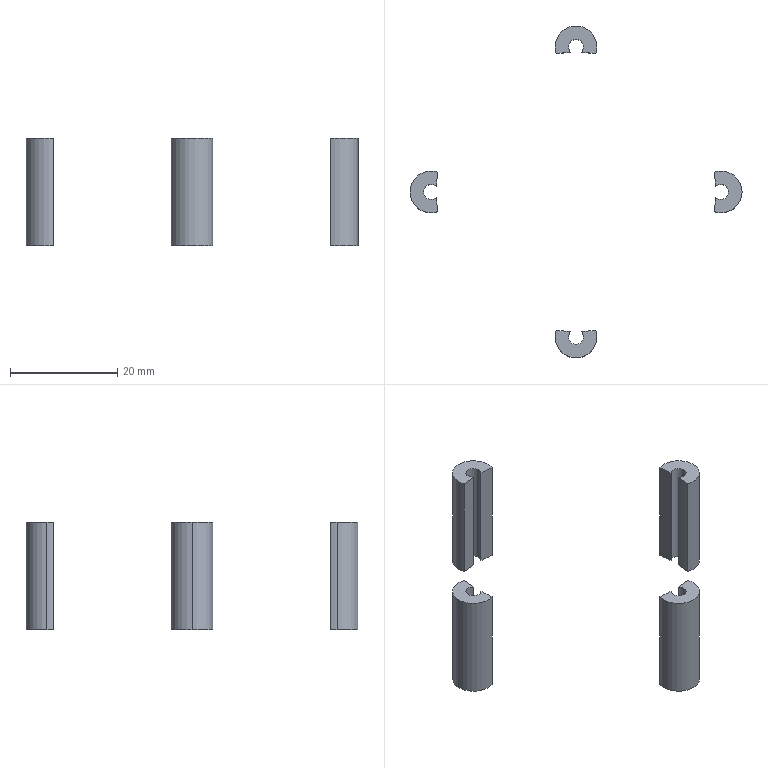Part | SolidWorks | features BaseBody 4 | 4 solids | 34 faces | box 61.8 x 61.8 x 20 mm | volume 2131 mm3 | cylinder 26 | plane 8 | commonest cylinder face diameters 2.8 x9 7.8 x9 52 x8
STEP:
#1=CARTESIAN_POINT('',(3.69,-25.737,11.));
#2=VERTEX_POINT('',#1);
#3=CARTESIAN_POINT('',(3.9,-27.,11.));
#4=VERTEX_POINT('',#3);
#5=CARTESIAN_POINT('',(0.,-27.,11.));
#6=DIRECTION('',(0.,0.,-1.));
#7=DIRECTION('',(-1.,0.,0.));
#8=AXIS2_PLACEMENT_3D('',#5,#6,#7);
#9=CIRCLE('',#8,3.9);
#10=EDGE_CURVE('',#2,#4,#9,.T.);
#11=ORIENTED_EDGE('',*,*,#10,.T.);
#12=CARTESIAN_POINT('',(3.9,-27.,-9.));
#13=VERTEX_POINT('',#12);
#14=CARTESIAN_POINT('',(3.9,-27.,-9.));
#15=DIRECTION('',(0.,0.,-1.));
#16=VECTOR('',#15,1000.);
#17=LINE('',#14,#16);
#18=EDGE_CURVE('',#4,#13,#17,.T.);
#19=ORIENTED_EDGE('',*,*,#18,.T.);
#20=CARTESIAN_POINT('',(3.69,-25.737,-9.));
#21=VERTEX_POINT('',#20);
#22=CARTESIAN_POINT('',(0.,-27.,-9.));
#23=DIRECTION('',(0.,0.,1.));
#24=DIRECTION('',(-1.,0.,0.));
#25=AXIS2_PLACEMENT_3D('',#22,#23,#24);
#26=CIRCLE('',#25,3.9);
#27=EDGE_CURVE('',#13,#21,#26,.T.);
#28=ORIENTED_EDGE('',*,*,#27,.T.);
#29=CARTESIAN_POINT('',(3.69,-25.737,-9.));
#30=DIRECTION('',(0.,0.,1.));
#31=VECTOR('',#30,1000.);
#32=LINE('',#29,#31);
#33=EDGE_CURVE('',#21,#2,#32,.T.);
#34=ORIENTED_EDGE('',*,*,#33,.T.);
#35=EDGE_LOOP('',(#11,#19,#28,#34));
#36=FACE_OUTER_BOUND('',#35,.T.);
#37=CARTESIAN_POINT('',(0.,-27.,-9.));
#38=DIRECTION('',(0.,0.,-1.));
#39=DIRECTION('',(-1.,0.,0.));
#40=AXIS2_PLACEMENT_3D('',#37,#38,#39);
#41=CYLINDRICAL_SURFACE('',#40,3.9);
#42=ADVANCED_FACE('',(#36),#41,.T.);
#43=ORIENTED_EDGE('',*,*,#18,.F.);
#44=CARTESIAN_POINT('',(-3.9,-27.,11.));
#45=VERTEX_POINT('',#44);
#46=CARTESIAN_POINT('',(0.,-27.,11.));
#47=DIRECTION('',(0.,0.,-1.));
#48=DIRECTION('',(-1.,0.,0.));
#49=AXIS2_PLACEMENT_3D('',#46,#47,#48);
#50=CIRCLE('',#49,3.9);
#51=EDGE_CURVE('',#4,#45,#50,.T.);
#52=ORIENTED_EDGE('',*,*,#51,.T.);
#53=CARTESIAN_POINT('',(-3.9,-27.,-9.));
#54=VERTEX_POINT('',#53);
#55=CARTESIAN_POINT('',(-3.9,-27.,-9.));
#56=DIRECTION('',(0.,0.,-1.));
#57=VECTOR('',#56,1000.);
#58=LINE('',#55,#57);
#59=EDGE_CURVE('',#45,#54,#58,.T.);
#60=ORIENTED_EDGE('',*,*,#59,.T.);
#61=CARTESIAN_POINT('',(0.,-27.,-9.));
#62=DIRECTION('',(0.,0.,1.));
#63=DIRECTION('',(-1.,0.,0.));
#64=AXIS2_PLACEMENT_3D('',#61,#62,#63);
#65=CIRCLE('',#64,3.9);
#66=EDGE_CURVE('',#54,#13,#65,.T.);
#67=ORIENTED_EDGE('',*,*,#66,.T.);
#68=EDGE_LOOP('',(#43,#52,#60,#67));
#69=FACE_OUTER_BOUND('',#68,.T.);
#70=CARTESIAN_POINT('',(0.,-27.,-9.));
#71=DIRECTION('',(0.,0.,-1.));
#72=DIRECTION('',(-1.,0.,0.));
#73=AXIS2_PLACEMENT_3D('',#70,#71,#72);
#74=CYLINDRICAL_SURFACE('',#73,3.9);
#75=ADVANCED_FACE('',(#69),#74,.T.);
#76=CARTESIAN_POINT('',(1.4,-27.,11.));
#77=VERTEX_POINT('',#76);
#78=CARTESIAN_POINT('',(-1.4,-27.,11.));
#79=VERTEX_POINT('',#78);
#80=CARTESIAN_POINT('',(0.,-27.,11.));
#81=DIRECTION('',(0.,0.,-1.));
#82=DIRECTION('',(-1.,0.,0.));
#83=AXIS2_PLACEMENT_3D('',#80,#81,#82);
#84=CIRCLE('',#83,1.4);
#85=EDGE_CURVE('',#77,#79,#84,.T.);
#86=ORIENTED_EDGE('',*,*,#85,.F.);
#87=CARTESIAN_POINT('',(1.4,-27.,-9.));
#88=VERTEX_POINT('',#87);
#89=CARTESIAN_POINT('',(1.4,-27.,-9.));
#90=DIRECTION('',(0.,0.,-1.));
#91=VECTOR('',#90,1000.);
#92=LINE('',#89,#91);
#93=EDGE_CURVE('',#77,#88,#92,.T.);
#94=ORIENTED_EDGE('',*,*,#93,.T.);
#95=CARTESIAN_POINT('',(-1.4,-27.,-9.));
#96=VERTEX_POINT('',#95);
#97=CARTESIAN_POINT('',(0.,-27.,-9.));
#98=DIRECTION('',(0.,0.,-1.));
#99=DIRECTION('',(-1.,0.,0.));
#100=AXIS2_PLACEMENT_3D('',#97,#98,#99);
#101=CIRCLE('',#100,1.4);
#102=EDGE_CURVE('',#88,#96,#101,.T.);
#103=ORIENTED_EDGE('',*,*,#102,.T.);
#104=CARTESIAN_POINT('',(-1.4,-27.,-9.));
#105=DIRECTION('',(0.,0.,-1.));
#106=VECTOR('',#105,1000.);
#107=LINE('',#104,#106);
#108=EDGE_CURVE('',#79,#96,#107,.T.);
#109=ORIENTED_EDGE('',*,*,#108,.F.);
#110=EDGE_LOOP('',(#86,#94,#103,#109));
#111=FACE_OUTER_BOUND('',#110,.T.);
#112=CARTESIAN_POINT('',(0.,-27.,-9.));
#113=DIRECTION('',(0.,0.,-1.));
#114=DIRECTION('',(-1.,0.,0.));
#115=AXIS2_PLACEMENT_3D('',#112,#113,#114);
#116=CYLINDRICAL_SURFACE('',#115,1.4);
#117=ADVANCED_FACE('',(#111),#116,.F.);
#118=CARTESIAN_POINT('',(-0.9613,-25.982,11.));
#119=VERTEX_POINT('',#118);
#120=CARTESIAN_POINT('',(0.,-27.,11.));
#121=DIRECTION('',(0.,0.,-1.));
#122=DIRECTION('',(-1.,0.,0.));
#123=AXIS2_PLACEMENT_3D('',#120,#121,#122);
#124=CIRCLE('',#123,1.4);
#125=EDGE_CURVE('',#79,#119,#124,.T.);
#126=ORIENTED_EDGE('',*,*,#125,.F.);
#127=ORIENTED_EDGE('',*,*,#108,.T.);
#128=CARTESIAN_POINT('',(-0.9613,-25.982,-9.));
#129=VERTEX_POINT('',#128);
#130=CARTESIAN_POINT('',(0.,-27.,-9.));
#131=DIRECTION('',(0.,0.,-1.));
#132=DIRECTION('',(-1.,0.,0.));
#133=AXIS2_PLACEMENT_3D('',#130,#131,#132);
#134=CIRCLE('',#133,1.4);
#135=EDGE_CURVE('',#96,#129,#134,.T.);
#136=ORIENTED_EDGE('',*,*,#135,.T.);
#137=CARTESIAN_POINT('',(-0.9613,-25.982,-9.));
#138=DIRECTION('',(0.,0.,1.));
#139=VECTOR('',#138,1000.);
#140=LINE('',#137,#139);
#141=EDGE_CURVE('',#129,#119,#140,.T.);
#142=ORIENTED_EDGE('',*,*,#141,.T.);
#143=EDGE_LOOP('',(#126,#127,#136,#142));
#144=FACE_OUTER_BOUND('',#143,.T.);
#145=CARTESIAN_POINT('',(0.,-27.,-9.));
#146=DIRECTION('',(0.,0.,-1.));
#147=DIRECTION('',(-1.,0.,0.));
#148=AXIS2_PLACEMENT_3D('',#145,#146,#147);
#149=CYLINDRICAL_SURFACE('',#148,1.4);
#150=ADVANCED_FACE('',(#144),#149,.F.);
#151=ORIENTED_EDGE('',*,*,#59,.F.);
#152=CARTESIAN_POINT('',(-3.69,-25.737,11.));
#153=VERTEX_POINT('',#152);
#154=CARTESIAN_POINT('',(0.,-27.,11.));
#155=DIRECTION('',(0.,0.,-1.));
#156=DIRECTION('',(-1.,0.,0.));
#157=AXIS2_PLACEMENT_3D('',#154,#155,#156);
#158=CIRCLE('',#157,3.9);
#159=EDGE_CURVE('',#45,#153,#158,.T.);
#160=ORIENTED_EDGE('',*,*,#159,.T.);
#161=CARTESIAN_POINT('',(-3.69,-25.737,-9.));
#162=VERTEX_POINT('',#161);
#163=CARTESIAN_POINT('',(-3.69,-25.737,-9.));
#164=DIRECTION('',(0.,0.,-1.));
#165=VECTOR('',#164,1000.);
#166=LINE('',#163,#165);
#167=EDGE_CURVE('',#153,#162,#166,.T.);
#168=ORIENTED_EDGE('',*,*,#167,.T.);
#169=CARTESIAN_POINT('',(0.,-27.,-9.));
#170=DIRECTION('',(0.,0.,1.));
#171=DIRECTION('',(-1.,0.,0.));
#172=AXIS2_PLACEMENT_3D('',#169,#170,#171);
#173=CIRCLE('',#172,3.9);
#174=EDGE_CURVE('',#162,#54,#173,.T.);
#175=ORIENTED_EDGE('',*,*,#174,.T.);
#176=EDGE_LOOP('',(#151,#160,#168,#175));
#177=FACE_OUTER_BOUND('',#176,.T.);
#178=CARTESIAN_POINT('',(0.,-27.,-9.));
#179=DIRECTION('',(0.,0.,-1.));
#180=DIRECTION('',(-1.,0.,0.));
#181=AXIS2_PLACEMENT_3D('',#178,#179,#180);
#182=CYLINDRICAL_SURFACE('',#181,3.9);
#183=ADVANCED_FACE('',(#177),#182,.T.);
#184=CARTESIAN_POINT('',(0.9613,-25.982,11.));
#185=VERTEX_POINT('',#184);
#186=CARTESIAN_POINT('',(0.,-27.,11.));
#187=DIRECTION('',(0.,0.,-1.));
#188=DIRECTION('',(-1.,0.,0.));
#189=AXIS2_PLACEMENT_3D('',#186,#187,#188);
#190=CIRCLE('',#189,1.4);
#191=EDGE_CURVE('',#185,#77,#190,.T.);
#192=ORIENTED_EDGE('',*,*,#191,.T.);
#193=ORIENTED_EDGE('',*,*,#85,.T.);
#194=ORIENTED_EDGE('',*,*,#125,.T.);
#195=CARTESIAN_POINT('',(0.,0.,11.));
#196=DIRECTION('',(0.,0.,-1.));
#197=DIRECTION('',(1.,0.,0.));
#198=AXIS2_PLACEMENT_3D('',#195,#196,#197);
#199=CIRCLE('',#198,26.);
#200=EDGE_CURVE('',#119,#153,#199,.T.);
#201=ORIENTED_EDGE('',*,*,#200,.T.);
#202=ORIENTED_EDGE('',*,*,#159,.F.);
#203=ORIENTED_EDGE('',*,*,#51,.F.);
#204=ORIENTED_EDGE('',*,*,#10,.F.);
#205=CARTESIAN_POINT('',(0.,0.,11.));
#206=DIRECTION('',(0.,0.,-1.));
#207=DIRECTION('',(1.,0.,0.));
#208=AXIS2_PLACEMENT_3D('',#205,#206,#207);
#209=CIRCLE('',#208,26.);
#210=EDGE_CURVE('',#2,#185,#209,.T.);
#211=ORIENTED_EDGE('',*,*,#210,.T.);
#212=EDGE_LOOP('',(#192,#193,#194,#201,#202,#203,#204,#211));
#213=FACE_OUTER_BOUND('',#212,.T.);
#214=CARTESIAN_POINT('',(0.,-30.9,11.));
#215=DIRECTION('',(0.,0.,1.));
#216=DIRECTION('',(1.,0.,0.));
#217=AXIS2_PLACEMENT_3D('',#214,#215,#216);
#218=PLANE('',#217);
#219=ADVANCED_FACE('',(#213),#218,.T.);
#220=CARTESIAN_POINT('',(0.9613,-25.982,-9.));
#221=VERTEX_POINT('',#220);
#222=CARTESIAN_POINT('',(0.,0.,-9.));
#223=DIRECTION('',(0.,0.,1.));
#224=DIRECTION('',(1.,0.,0.));
#225=AXIS2_PLACEMENT_3D('',#222,#223,#224);
#226=CIRCLE('',#225,26.);
#227=EDGE_CURVE('',#221,#21,#226,.T.);
#228=ORIENTED_EDGE('',*,*,#227,.F.);
#229=CARTESIAN_POINT('',(0.9613,-25.982,-9.));
#230=DIRECTION('',(0.,0.,-1.));
#231=VECTOR('',#230,1000.);
#232=LINE('',#229,#231);
#233=EDGE_CURVE('',#185,#221,#232,.T.);
#234=ORIENTED_EDGE('',*,*,#233,.F.);
#235=ORIENTED_EDGE('',*,*,#210,.F.);
#236=ORIENTED_EDGE('',*,*,#33,.F.);
#237=EDGE_LOOP('',(#228,#234,#235,#236));
#238=FACE_OUTER_BOUND('',#237,.T.);
#239=CARTESIAN_POINT('',(0.,0.,-9.));
#240=DIRECTION('',(0.,0.,1.));
#241=DIRECTION('',(1.,0.,0.));
#242=AXIS2_PLACEMENT_3D('',#239,#240,#241);
#243=CYLINDRICAL_SURFACE('',#242,26.);
#244=ADVANCED_FACE('',(#238),#243,.F.);
#245=CARTESIAN_POINT('',(0.,-27.,-9.));
#246=DIRECTION('',(0.,0.,-1.));
#247=DIRECTION('',(-1.,0.,0.));
#248=AXIS2_PLACEMENT_3D('',#245,#246,#247);
#249=CIRCLE('',#248,1.4);
#250=EDGE_CURVE('',#221,#88,#249,.T.);
#251=ORIENTED_EDGE('',*,*,#250,.F.);
#252=ORIENTED_EDGE('',*,*,#227,.T.);
#253=ORIENTED_EDGE('',*,*,#27,.F.);
#254=ORIENTED_EDGE('',*,*,#66,.F.);
#255=ORIENTED_EDGE('',*,*,#174,.F.);
#256=CARTESIAN_POINT('',(0.,0.,-9.));
#257=DIRECTION('',(0.,0.,-1.));
#258=DIRECTION('',(1.,0.,0.));
#259=AXIS2_PLACEMENT_3D('',#256,#257,#258);
#260=CIRCLE('',#259,26.);
#261=EDGE_CURVE('',#129,#162,#260,.T.);
#262=ORIENTED_EDGE('',*,*,#261,.F.);
#263=ORIENTED_EDGE('',*,*,#135,.F.);
#264=ORIENTED_EDGE('',*,*,#102,.F.);
#265=EDGE_LOOP('',(#251,#252,#253,#254,#255,#262,#263,#264));
#266=FACE_OUTER_BOUND('',#265,.T.);
#267=CARTESIAN_POINT('',(0.,-30.9,-9.));
#268=DIRECTION('',(0.,0.,1.));
#269=DIRECTION('',(1.,0.,0.));
#270=AXIS2_PLACEMENT_3D('',#267,#268,#269);
#271=PLANE('',#270);
#272=ADVANCED_FACE('',(#266),#271,.F.);
#273=ORIENTED_EDGE('',*,*,#261,.T.);
#274=ORIENTED_EDGE('',*,*,#167,.F.);
#275=ORIENTED_EDGE('',*,*,#200,.F.);
#276=ORIENTED_EDGE('',*,*,#141,.F.);
#277=EDGE_LOOP('',(#273,#274,#275,#276));
#278=FACE_OUTER_BOUND('',#277,.T.);
#279=CARTESIAN_POINT('',(0.,0.,-9.));
#280=DIRECTION('',(0.,0.,1.));
#281=DIRECTION('',(1.,0.,0.));
#282=AXIS2_PLACEMENT_3D('',#279,#280,#281);
#283=CYLINDRICAL_SURFACE('',#282,26.);
#284=ADVANCED_FACE('',(#278),#283,.F.);
#285=ORIENTED_EDGE('',*,*,#93,.F.);
#286=ORIENTED_EDGE('',*,*,#191,.F.);
#287=ORIENTED_EDGE('',*,*,#233,.T.);
#288=ORIENTED_EDGE('',*,*,#250,.T.);
#289=EDGE_LOOP('',(#285,#286,#287,#288));
#290=FACE_OUTER_BOUND('',#289,.T.);
#291=CARTESIAN_POINT('',(0.,-27.,-9.));
#292=DIRECTION('',(0.,0.,-1.));
#293=DIRECTION('',(-1.,0.,0.));
#294=AXIS2_PLACEMENT_3D('',#291,#292,#293);
#295=CYLINDRICAL_SURFACE('',#294,1.4);
#296=ADVANCED_FACE('',(#290),#295,.F.);
#297=CLOSED_SHELL('',(#42,#75,#117,#150,#183,#219,#244,#272,#284,#296));
#298=MANIFOLD_SOLID_BREP('',#297);
#299=CARTESIAN_POINT('',(-3.9,27.,11.));
#300=VERTEX_POINT('',#299);
#301=CARTESIAN_POINT('',(3.9,27.,11.));
#302=VERTEX_POINT('',#301);
#303=CARTESIAN_POINT('',(0.,27.,11.));
#304=DIRECTION('',(0.,0.,-1.));
#305=DIRECTION('',(-1.,0.,0.));
#306=AXIS2_PLACEMENT_3D('',#303,#304,#305);
#307=CIRCLE('',#306,3.9);
#308=EDGE_CURVE('',#300,#302,#307,.T.);
#309=ORIENTED_EDGE('',*,*,#308,.T.);
#310=CARTESIAN_POINT('',(3.9,27.,-9.));
#311=VERTEX_POINT('',#310);
#312=CARTESIAN_POINT('',(3.9,27.,-9.));
#313=DIRECTION('',(0.,0.,-1.));
#314=VECTOR('',#313,1000.);
#315=LINE('',#312,#314);
#316=EDGE_CURVE('',#302,#311,#315,.T.);
#317=ORIENTED_EDGE('',*,*,#316,.T.);
#318=CARTESIAN_POINT('',(-3.9,27.,-9.));
#319=VERTEX_POINT('',#318);
#320=CARTESIAN_POINT('',(0.,27.,-9.));
#321=DIRECTION('',(0.,0.,1.));
#322=DIRECTION('',(-1.,0.,0.));
#323=AXIS2_PLACEMENT_3D('',#320,#321,#322);
#324=CIRCLE('',#323,3.9);
#325=EDGE_CURVE('',#311,#319,#324,.T.);
#326=ORIENTED_EDGE('',*,*,#325,.T.);
#327=CARTESIAN_POINT('',(-3.9,27.,-9.));
#328=DIRECTION('',(0.,0.,-1.));
#329=VECTOR('',#328,1000.);
#330=LINE('',#327,#329);
#331=EDGE_CURVE('',#300,#319,#330,.T.);
#332=ORIENTED_EDGE('',*,*,#331,.F.);
#333=EDGE_LOOP('',(#309,#317,#326,#332));
#334=FACE_OUTER_BOUND('',#333,.T.);
#335=CARTESIAN_POINT('',(0.,27.,-9.));
#336=DIRECTION('',(0.,0.,-1.));
#337=DIRECTION('',(-1.,0.,0.));
#338=AXIS2_PLACEMENT_3D('',#335,#336,#337);
#339=CYLINDRICAL_SURFACE('',#338,3.9);
#340=ADVANCED_FACE('',(#334),#339,.T.);
#341=CARTESIAN_POINT('',(-3.69,25.737,11.));
#342=VERTEX_POINT('',#341);
#343=CARTESIAN_POINT('',(0.,27.,11.));
#344=DIRECTION('',(0.,0.,-1.));
#345=DIRECTION('',(-1.,0.,0.));
#346=AXIS2_PLACEMENT_3D('',#343,#344,#345);
#347=CIRCLE('',#346,3.9);
#348=EDGE_CURVE('',#342,#300,#347,.T.);
#349=ORIENTED_EDGE('',*,*,#348,.T.);
#350=ORIENTED_EDGE('',*,*,#331,.T.);
#351=CARTESIAN_POINT('',(-3.69,25.737,-9.));
#352=VERTEX_POINT('',#351);
#353=CARTESIAN_POINT('',(0.,27.,-9.));
#354=DIRECTION('',(0.,0.,1.));
#355=DIRECTION('',(-1.,0.,0.));
#356=AXIS2_PLACEMENT_3D('',#353,#354,#355);
#357=CIRCLE('',#356,3.9);
#358=EDGE_CURVE('',#319,#352,#357,.T.);
#359=ORIENTED_EDGE('',*,*,#358,.T.);
#360=CARTESIAN_POINT('',(-3.69,25.737,-9.));
#361=DIRECTION('',(0.,0.,1.));
#362=VECTOR('',#361,1000.);
#363=LINE('',#360,#362);
#364=EDGE_CURVE('',#352,#342,#363,.T.);
#365=ORIENTED_EDGE('',*,*,#364,.T.);
#366=EDGE_LOOP('',(#349,#350,#359,#365));
#367=FACE_OUTER_BOUND('',#366,.T.);
#368=CARTESIAN_POINT('',(0.,27.,-9.));
#369=DIRECTION('',(0.,0.,-1.));
#370=DIRECTION('',(-1.,0.,0.));
#371=AXIS2_PLACEMENT_3D('',#368,#369,#370);
#372=CYLINDRICAL_SURFACE('',#371,3.9);
#373=ADVANCED_FACE('',(#367),#372,.T.);
#374=CARTESIAN_POINT('',(1.4,27.,11.));
#375=VERTEX_POINT('',#374);
#376=CARTESIAN_POINT('',(0.9613,25.982,11.));
#377=VERTEX_POINT('',#376);
#378=CARTESIAN_POINT('',(0.,27.,11.));
#379=DIRECTION('',(0.,0.,-1.));
#380=DIRECTION('',(-1.,0.,0.));
#381=AXIS2_PLACEMENT_3D('',#378,#379,#380);
#382=CIRCLE('',#381,1.4);
#383=EDGE_CURVE('',#375,#377,#382,.T.);
#384=ORIENTED_EDGE('',*,*,#383,.F.);
#385=CARTESIAN_POINT('',(1.4,27.,-9.));
#386=VERTEX_POINT('',#385);
#387=CARTESIAN_POINT('',(1.4,27.,-9.));
#388=DIRECTION('',(0.,0.,-1.));
#389=VECTOR('',#388,1000.);
#390=LINE('',#387,#389);
#391=EDGE_CURVE('',#375,#386,#390,.T.);
#392=ORIENTED_EDGE('',*,*,#391,.T.);
#393=CARTESIAN_POINT('',(0.9613,25.982,-9.));
#394=VERTEX_POINT('',#393);
#395=CARTESIAN_POINT('',(0.,27.,-9.));
#396=DIRECTION('',(0.,0.,-1.));
#397=DIRECTION('',(-1.,0.,0.));
#398=AXIS2_PLACEMENT_3D('',#395,#396,#397);
#399=CIRCLE('',#398,1.4);
#400=EDGE_CURVE('',#386,#394,#399,.T.);
#401=ORIENTED_EDGE('',*,*,#400,.T.);
#402=CARTESIAN_POINT('',(0.9613,25.982,-9.));
#403=DIRECTION('',(0.,0.,1.));
#404=VECTOR('',#403,1000.);
#405=LINE('',#402,#404);
#406=EDGE_CURVE('',#394,#377,#405,.T.);
#407=ORIENTED_EDGE('',*,*,#406,.T.);
#408=EDGE_LOOP('',(#384,#392,#401,#407));
#409=FACE_OUTER_BOUND('',#408,.T.);
#410=CARTESIAN_POINT('',(0.,27.,-9.));
#411=DIRECTION('',(0.,0.,-1.));
#412=DIRECTION('',(-1.,0.,0.));
#413=AXIS2_PLACEMENT_3D('',#410,#411,#412);
#414=CYLINDRICAL_SURFACE('',#413,1.4);
#415=ADVANCED_FACE('',(#409),#414,.F.);
#416=ORIENTED_EDGE('',*,*,#391,.F.);
#417=CARTESIAN_POINT('',(-1.4,27.,11.));
#418=VERTEX_POINT('',#417);
#419=CARTESIAN_POINT('',(0.,27.,11.));
#420=DIRECTION('',(0.,0.,-1.));
#421=DIRECTION('',(-1.,0.,0.));
#422=AXIS2_PLACEMENT_3D('',#419,#420,#421);
#423=CIRCLE('',#422,1.4);
#424=EDGE_CURVE('',#418,#375,#423,.T.);
#425=ORIENTED_EDGE('',*,*,#424,.F.);
#426=CARTESIAN_POINT('',(-1.4,27.,-9.));
#427=VERTEX_POINT('',#426);
#428=CARTESIAN_POINT('',(-1.4,27.,-9.));
#429=DIRECTION('',(0.,0.,-1.));
#430=VECTOR('',#429,1000.);
#431=LINE('',#428,#430);
#432=EDGE_CURVE('',#418,#427,#431,.T.);
#433=ORIENTED_EDGE('',*,*,#432,.T.);
#434=CARTESIAN_POINT('',(0.,27.,-9.));
#435=DIRECTION('',(0.,0.,-1.));
#436=DIRECTION('',(-1.,0.,0.));
#437=AXIS2_PLACEMENT_3D('',#434,#435,#436);
#438=CIRCLE('',#437,1.4);
#439=EDGE_CURVE('',#427,#386,#438,.T.);
#440=ORIENTED_EDGE('',*,*,#439,.T.);
#441=EDGE_LOOP('',(#416,#425,#433,#440));
#442=FACE_OUTER_BOUND('',#441,.T.);
#443=CARTESIAN_POINT('',(0.,27.,-9.));
#444=DIRECTION('',(0.,0.,-1.));
#445=DIRECTION('',(-1.,0.,0.));
#446=AXIS2_PLACEMENT_3D('',#443,#444,#445);
#447=CYLINDRICAL_SURFACE('',#446,1.4);
#448=ADVANCED_FACE('',(#442),#447,.F.);
#449=ORIENTED_EDGE('',*,*,#316,.F.);
#450=CARTESIAN_POINT('',(3.69,25.737,11.));
#451=VERTEX_POINT('',#450);
#452=CARTESIAN_POINT('',(0.,27.,11.));
#453=DIRECTION('',(0.,0.,-1.));
#454=DIRECTION('',(-1.,0.,0.));
#455=AXIS2_PLACEMENT_3D('',#452,#453,#454);
#456=CIRCLE('',#455,3.9);
#457=EDGE_CURVE('',#302,#451,#456,.T.);
#458=ORIENTED_EDGE('',*,*,#457,.T.);
#459=CARTESIAN_POINT('',(3.69,25.737,-9.));
#460=VERTEX_POINT('',#459);
#461=CARTESIAN_POINT('',(3.69,25.737,-9.));
#462=DIRECTION('',(0.,0.,-1.));
#463=VECTOR('',#462,1000.);
#464=LINE('',#461,#463);
#465=EDGE_CURVE('',#451,#460,#464,.T.);
#466=ORIENTED_EDGE('',*,*,#465,.T.);
#467=CARTESIAN_POINT('',(0.,27.,-9.));
#468=DIRECTION('',(0.,0.,1.));
#469=DIRECTION('',(-1.,0.,0.));
#470=AXIS2_PLACEMENT_3D('',#467,#468,#469);
#471=CIRCLE('',#470,3.9);
#472=EDGE_CURVE('',#460,#311,#471,.T.);
#473=ORIENTED_EDGE('',*,*,#472,.T.);
#474=EDGE_LOOP('',(#449,#458,#466,#473));
#475=FACE_OUTER_BOUND('',#474,.T.);
#476=CARTESIAN_POINT('',(0.,27.,-9.));
#477=DIRECTION('',(0.,0.,-1.));
#478=DIRECTION('',(-1.,0.,0.));
#479=AXIS2_PLACEMENT_3D('',#476,#477,#478);
#480=CYLINDRICAL_SURFACE('',#479,3.9);
#481=ADVANCED_FACE('',(#475),#480,.T.);
#482=CARTESIAN_POINT('',(-0.9613,25.982,11.));
#483=VERTEX_POINT('',#482);
#484=CARTESIAN_POINT('',(0.,27.,11.));
#485=DIRECTION('',(0.,0.,-1.));
#486=DIRECTION('',(-1.,0.,0.));
#487=AXIS2_PLACEMENT_3D('',#484,#485,#486);
#488=CIRCLE('',#487,1.4);
#489=EDGE_CURVE('',#483,#418,#488,.T.);
#490=ORIENTED_EDGE('',*,*,#489,.T.);
#491=ORIENTED_EDGE('',*,*,#424,.T.);
#492=ORIENTED_EDGE('',*,*,#383,.T.);
#493=CARTESIAN_POINT('',(0.,0.,11.));
#494=DIRECTION('',(0.,0.,-1.));
#495=DIRECTION('',(1.,0.,0.));
#496=AXIS2_PLACEMENT_3D('',#493,#494,#495);
#497=CIRCLE('',#496,26.);
#498=EDGE_CURVE('',#377,#451,#497,.T.);
#499=ORIENTED_EDGE('',*,*,#498,.T.);
#500=ORIENTED_EDGE('',*,*,#457,.F.);
#501=ORIENTED_EDGE('',*,*,#308,.F.);
#502=ORIENTED_EDGE('',*,*,#348,.F.);
#503=CARTESIAN_POINT('',(0.,0.,11.));
#504=DIRECTION('',(0.,0.,-1.));
#505=DIRECTION('',(1.,0.,0.));
#506=AXIS2_PLACEMENT_3D('',#503,#504,#505);
#507=CIRCLE('',#506,26.);
#508=EDGE_CURVE('',#342,#483,#507,.T.);
#509=ORIENTED_EDGE('',*,*,#508,.T.);
#510=EDGE_LOOP('',(#490,#491,#492,#499,#500,#501,#502,#509));
#511=FACE_OUTER_BOUND('',#510,.T.);
#512=CARTESIAN_POINT('',(0.,30.9,11.));
#513=DIRECTION('',(0.,0.,1.));
#514=DIRECTION('',(1.,0.,0.));
#515=AXIS2_PLACEMENT_3D('',#512,#513,#514);
#516=PLANE('',#515);
#517=ADVANCED_FACE('',(#511),#516,.T.);
#518=CARTESIAN_POINT('',(-0.9613,25.982,-9.));
#519=VERTEX_POINT('',#518);
#520=CARTESIAN_POINT('',(0.,0.,-9.));
#521=DIRECTION('',(0.,0.,1.));
#522=DIRECTION('',(1.,0.,0.));
#523=AXIS2_PLACEMENT_3D('',#520,#521,#522);
#524=CIRCLE('',#523,26.);
#525=EDGE_CURVE('',#519,#352,#524,.T.);
#526=ORIENTED_EDGE('',*,*,#525,.F.);
#527=CARTESIAN_POINT('',(-0.9613,25.982,-9.));
#528=DIRECTION('',(0.,0.,-1.));
#529=VECTOR('',#528,1000.);
#530=LINE('',#527,#529);
#531=EDGE_CURVE('',#483,#519,#530,.T.);
#532=ORIENTED_EDGE('',*,*,#531,.F.);
#533=ORIENTED_EDGE('',*,*,#508,.F.);
#534=ORIENTED_EDGE('',*,*,#364,.F.);
#535=EDGE_LOOP('',(#526,#532,#533,#534));
#536=FACE_OUTER_BOUND('',#535,.T.);
#537=CARTESIAN_POINT('',(0.,0.,-9.));
#538=DIRECTION('',(0.,0.,1.));
#539=DIRECTION('',(1.,0.,0.));
#540=AXIS2_PLACEMENT_3D('',#537,#538,#539);
#541=CYLINDRICAL_SURFACE('',#540,26.);
#542=ADVANCED_FACE('',(#536),#541,.F.);
#543=CARTESIAN_POINT('',(0.,27.,-9.));
#544=DIRECTION('',(0.,0.,-1.));
#545=DIRECTION('',(-1.,0.,0.));
#546=AXIS2_PLACEMENT_3D('',#543,#544,#545);
#547=CIRCLE('',#546,1.4);
#548=EDGE_CURVE('',#519,#427,#547,.T.);
#549=ORIENTED_EDGE('',*,*,#548,.F.);
#550=ORIENTED_EDGE('',*,*,#525,.T.);
#551=ORIENTED_EDGE('',*,*,#358,.F.);
#552=ORIENTED_EDGE('',*,*,#325,.F.);
#553=ORIENTED_EDGE('',*,*,#472,.F.);
#554=CARTESIAN_POINT('',(0.,0.,-9.));
#555=DIRECTION('',(0.,0.,-1.));
#556=DIRECTION('',(1.,0.,0.));
#557=AXIS2_PLACEMENT_3D('',#554,#555,#556);
#558=CIRCLE('',#557,26.);
#559=EDGE_CURVE('',#394,#460,#558,.T.);
#560=ORIENTED_EDGE('',*,*,#559,.F.);
#561=ORIENTED_EDGE('',*,*,#400,.F.);
#562=ORIENTED_EDGE('',*,*,#439,.F.);
#563=EDGE_LOOP('',(#549,#550,#551,#552,#553,#560,#561,#562));
#564=FACE_OUTER_BOUND('',#563,.T.);
#565=CARTESIAN_POINT('',(0.,30.9,-9.));
#566=DIRECTION('',(0.,0.,1.));
#567=DIRECTION('',(1.,0.,0.));
#568=AXIS2_PLACEMENT_3D('',#565,#566,#567);
#569=PLANE('',#568);
#570=ADVANCED_FACE('',(#564),#569,.F.);
#571=ORIENTED_EDGE('',*,*,#559,.T.);
#572=ORIENTED_EDGE('',*,*,#465,.F.);
#573=ORIENTED_EDGE('',*,*,#498,.F.);
#574=ORIENTED_EDGE('',*,*,#406,.F.);
#575=EDGE_LOOP('',(#571,#572,#573,#574));
#576=FACE_OUTER_BOUND('',#575,.T.);
#577=CARTESIAN_POINT('',(0.,0.,-9.));
#578=DIRECTION('',(0.,0.,1.));
#579=DIRECTION('',(1.,0.,0.));
#580=AXIS2_PLACEMENT_3D('',#577,#578,#579);
#581=CYLINDRICAL_SURFACE('',#580,26.);
#582=ADVANCED_FACE('',(#576),#581,.F.);
#583=ORIENTED_EDGE('',*,*,#432,.F.);
#584=ORIENTED_EDGE('',*,*,#489,.F.);
#585=ORIENTED_EDGE('',*,*,#531,.T.);
#586=ORIENTED_EDGE('',*,*,#548,.T.);
#587=EDGE_LOOP('',(#583,#584,#585,#586));
#588=FACE_OUTER_BOUND('',#587,.T.);
#589=CARTESIAN_POINT('',(0.,27.,-9.));
#590=DIRECTION('',(0.,0.,-1.));
#591=DIRECTION('',(-1.,0.,0.));
#592=AXIS2_PLACEMENT_3D('',#589,#590,#591);
#593=CYLINDRICAL_SURFACE('',#592,1.4);
#594=ADVANCED_FACE('',(#588),#593,.F.);
#595=CLOSED_SHELL('',(#340,#373,#415,#448,#481,#517,#542,#570,#582,#594));
#596=MANIFOLD_SOLID_BREP('',#595);
#597=CARTESIAN_POINT('',(25.737,3.69,11.));
#598=VERTEX_POINT('',#597);
#599=CARTESIAN_POINT('',(25.737,-3.69,11.));
#600=VERTEX_POINT('',#599);
#601=CARTESIAN_POINT('',(27.,0.,11.));
#602=DIRECTION('',(0.,0.,-1.));
#603=DIRECTION('',(-1.,0.,0.));
#604=AXIS2_PLACEMENT_3D('',#601,#602,#603);
#605=CIRCLE('',#604,3.9);
#606=EDGE_CURVE('',#598,#600,#605,.T.);
#607=ORIENTED_EDGE('',*,*,#606,.T.);
#608=CARTESIAN_POINT('',(25.737,-3.69,-9.));
#609=VERTEX_POINT('',#608);
#610=CARTESIAN_POINT('',(25.737,-3.69,-9.));
#611=DIRECTION('',(0.,0.,-1.));
#612=VECTOR('',#611,1000.);
#613=LINE('',#610,#612);
#614=EDGE_CURVE('',#600,#609,#613,.T.);
#615=ORIENTED_EDGE('',*,*,#614,.T.);
#616=CARTESIAN_POINT('',(25.737,3.69,-9.));
#617=VERTEX_POINT('',#616);
#618=CARTESIAN_POINT('',(27.,0.,-9.));
#619=DIRECTION('',(0.,0.,1.));
#620=DIRECTION('',(-1.,0.,0.));
#621=AXIS2_PLACEMENT_3D('',#618,#619,#620);
#622=CIRCLE('',#621,3.9);
#623=EDGE_CURVE('',#609,#617,#622,.T.);
#624=ORIENTED_EDGE('',*,*,#623,.T.);
#625=CARTESIAN_POINT('',(25.737,3.69,-9.));
#626=DIRECTION('',(0.,0.,1.));
#627=VECTOR('',#626,1000.);
#628=LINE('',#625,#627);
#629=EDGE_CURVE('',#617,#598,#628,.T.);
#630=ORIENTED_EDGE('',*,*,#629,.T.);
#631=EDGE_LOOP('',(#607,#615,#624,#630));
#632=FACE_OUTER_BOUND('',#631,.T.);
#633=CARTESIAN_POINT('',(27.,0.,-9.));
#634=DIRECTION('',(0.,0.,-1.));
#635=DIRECTION('',(-1.,0.,0.));
#636=AXIS2_PLACEMENT_3D('',#633,#634,#635);
#637=CYLINDRICAL_SURFACE('',#636,3.9);
#638=ADVANCED_FACE('',(#632),#637,.T.);
#639=CARTESIAN_POINT('',(25.982,-0.9613,-9.));
#640=VERTEX_POINT('',#639);
#641=CARTESIAN_POINT('',(0.,0.,-9.));
#642=DIRECTION('',(0.,0.,1.));
#643=DIRECTION('',(1.,0.,0.));
#644=AXIS2_PLACEMENT_3D('',#641,#642,#643);
#645=CIRCLE('',#644,26.);
#646=EDGE_CURVE('',#609,#640,#645,.T.);
#647=ORIENTED_EDGE('',*,*,#646,.F.);
#648=ORIENTED_EDGE('',*,*,#614,.F.);
#649=CARTESIAN_POINT('',(25.982,-0.9613,11.));
#650=VERTEX_POINT('',#649);
#651=CARTESIAN_POINT('',(0.,0.,11.));
#652=DIRECTION('',(0.,0.,-1.));
#653=DIRECTION('',(1.,0.,0.));
#654=AXIS2_PLACEMENT_3D('',#651,#652,#653);
#655=CIRCLE('',#654,26.);
#656=EDGE_CURVE('',#650,#600,#655,.T.);
#657=ORIENTED_EDGE('',*,*,#656,.F.);
#658=CARTESIAN_POINT('',(25.982,-0.9613,-9.));
#659=DIRECTION('',(0.,0.,1.));
#660=VECTOR('',#659,1000.);
#661=LINE('',#658,#660);
#662=EDGE_CURVE('',#640,#650,#661,.T.);
#663=ORIENTED_EDGE('',*,*,#662,.F.);
#664=EDGE_LOOP('',(#647,#648,#657,#663));
#665=FACE_OUTER_BOUND('',#664,.T.);
#666=CARTESIAN_POINT('',(0.,0.,-9.));
#667=DIRECTION('',(0.,0.,1.));
#668=DIRECTION('',(1.,0.,0.));
#669=AXIS2_PLACEMENT_3D('',#666,#667,#668);
#670=CYLINDRICAL_SURFACE('',#669,26.);
#671=ADVANCED_FACE('',(#665),#670,.F.);
#672=CARTESIAN_POINT('',(25.982,0.9613,11.));
#673=VERTEX_POINT('',#672);
#674=CARTESIAN_POINT('',(27.,0.,11.));
#675=DIRECTION('',(0.,0.,-1.));
#676=DIRECTION('',(-1.,0.,0.));
#677=AXIS2_PLACEMENT_3D('',#674,#675,#676);
#678=CIRCLE('',#677,1.4);
#679=EDGE_CURVE('',#673,#650,#678,.T.);
#680=ORIENTED_EDGE('',*,*,#679,.T.);
#681=ORIENTED_EDGE('',*,*,#656,.T.);
#682=ORIENTED_EDGE('',*,*,#606,.F.);
#683=CARTESIAN_POINT('',(0.,0.,11.));
#684=DIRECTION('',(0.,0.,-1.));
#685=DIRECTION('',(1.,0.,0.));
#686=AXIS2_PLACEMENT_3D('',#683,#684,#685);
#687=CIRCLE('',#686,26.);
#688=EDGE_CURVE('',#598,#673,#687,.T.);
#689=ORIENTED_EDGE('',*,*,#688,.T.);
#690=EDGE_LOOP('',(#680,#681,#682,#689));
#691=FACE_OUTER_BOUND('',#690,.T.);
#692=CARTESIAN_POINT('',(30.9,0.,11.));
#693=DIRECTION('',(0.,0.,1.));
#694=DIRECTION('',(1.,0.,0.));
#695=AXIS2_PLACEMENT_3D('',#692,#693,#694);
#696=PLANE('',#695);
#697=ADVANCED_FACE('',(#691),#696,.T.);
#698=CARTESIAN_POINT('',(25.982,0.9613,-9.));
#699=VERTEX_POINT('',#698);
#700=CARTESIAN_POINT('',(27.,0.,-9.));
#701=DIRECTION('',(0.,0.,-1.));
#702=DIRECTION('',(-1.,0.,0.));
#703=AXIS2_PLACEMENT_3D('',#700,#701,#702);
#704=CIRCLE('',#703,1.4);
#705=EDGE_CURVE('',#699,#640,#704,.T.);
#706=ORIENTED_EDGE('',*,*,#705,.F.);
#707=CARTESIAN_POINT('',(0.,0.,-9.));
#708=DIRECTION('',(0.,0.,-1.));
#709=DIRECTION('',(1.,0.,0.));
#710=AXIS2_PLACEMENT_3D('',#707,#708,#709);
#711=CIRCLE('',#710,26.);
#712=EDGE_CURVE('',#617,#699,#711,.T.);
#713=ORIENTED_EDGE('',*,*,#712,.F.);
#714=ORIENTED_EDGE('',*,*,#623,.F.);
#715=ORIENTED_EDGE('',*,*,#646,.T.);
#716=EDGE_LOOP('',(#706,#713,#714,#715));
#717=FACE_OUTER_BOUND('',#716,.T.);
#718=CARTESIAN_POINT('',(30.9,0.,-9.));
#719=DIRECTION('',(0.,0.,1.));
#720=DIRECTION('',(1.,0.,0.));
#721=AXIS2_PLACEMENT_3D('',#718,#719,#720);
#722=PLANE('',#721);
#723=ADVANCED_FACE('',(#717),#722,.F.);
#724=ORIENTED_EDGE('',*,*,#679,.F.);
#725=CARTESIAN_POINT('',(25.982,0.9613,-9.));
#726=DIRECTION('',(0.,0.,1.));
#727=VECTOR('',#726,1000.);
#728=LINE('',#725,#727);
#729=EDGE_CURVE('',#699,#673,#728,.T.);
#730=ORIENTED_EDGE('',*,*,#729,.F.);
#731=ORIENTED_EDGE('',*,*,#705,.T.);
#732=ORIENTED_EDGE('',*,*,#662,.T.);
#733=EDGE_LOOP('',(#724,#730,#731,#732));
#734=FACE_OUTER_BOUND('',#733,.T.);
#735=CARTESIAN_POINT('',(27.,0.,-9.));
#736=DIRECTION('',(0.,0.,-1.));
#737=DIRECTION('',(-1.,0.,0.));
#738=AXIS2_PLACEMENT_3D('',#735,#736,#737);
#739=CYLINDRICAL_SURFACE('',#738,1.4);
#740=ADVANCED_FACE('',(#734),#739,.F.);
#741=ORIENTED_EDGE('',*,*,#712,.T.);
#742=ORIENTED_EDGE('',*,*,#729,.T.);
#743=ORIENTED_EDGE('',*,*,#688,.F.);
#744=ORIENTED_EDGE('',*,*,#629,.F.);
#745=EDGE_LOOP('',(#741,#742,#743,#744));
#746=FACE_OUTER_BOUND('',#745,.T.);
#747=CARTESIAN_POINT('',(0.,0.,-9.));
#748=DIRECTION('',(0.,0.,1.));
#749=DIRECTION('',(1.,0.,0.));
#750=AXIS2_PLACEMENT_3D('',#747,#748,#749);
#751=CYLINDRICAL_SURFACE('',#750,26.);
#752=ADVANCED_FACE('',(#746),#751,.F.);
#753=CLOSED_SHELL('',(#638,#671,#697,#723,#740,#752));
#754=MANIFOLD_SOLID_BREP('',#753);
#755=CARTESIAN_POINT('',(-25.737,-3.69,11.));
#756=VERTEX_POINT('',#755);
#757=CARTESIAN_POINT('',(-30.9,0.,11.));
#758=VERTEX_POINT('',#757);
#759=CARTESIAN_POINT('',(-27.,0.,11.));
#760=DIRECTION('',(0.,0.,-1.));
#761=DIRECTION('',(-1.,0.,0.));
#762=AXIS2_PLACEMENT_3D('',#759,#760,#761);
#763=CIRCLE('',#762,3.9);
#764=EDGE_CURVE('',#756,#758,#763,.T.);
#765=ORIENTED_EDGE('',*,*,#764,.T.);
#766=CARTESIAN_POINT('',(-30.9,0.,-9.));
#767=VERTEX_POINT('',#766);
#768=CARTESIAN_POINT('',(-30.9,0.,-9.));
#769=DIRECTION('',(0.,0.,-1.));
#770=VECTOR('',#769,1000.);
#771=LINE('',#768,#770);
#772=EDGE_CURVE('',#758,#767,#771,.T.);
#773=ORIENTED_EDGE('',*,*,#772,.T.);
#774=CARTESIAN_POINT('',(-25.737,-3.69,-9.));
#775=VERTEX_POINT('',#774);
#776=CARTESIAN_POINT('',(-27.,0.,-9.));
#777=DIRECTION('',(0.,0.,1.));
#778=DIRECTION('',(-1.,0.,0.));
#779=AXIS2_PLACEMENT_3D('',#776,#777,#778);
#780=CIRCLE('',#779,3.9);
#781=EDGE_CURVE('',#767,#775,#780,.T.);
#782=ORIENTED_EDGE('',*,*,#781,.T.);
#783=CARTESIAN_POINT('',(-25.737,-3.69,-9.));
#784=DIRECTION('',(0.,0.,1.));
#785=VECTOR('',#784,1000.);
#786=LINE('',#783,#785);
#787=EDGE_CURVE('',#775,#756,#786,.T.);
#788=ORIENTED_EDGE('',*,*,#787,.T.);
#789=EDGE_LOOP('',(#765,#773,#782,#788));
#790=FACE_OUTER_BOUND('',#789,.T.);
#791=CARTESIAN_POINT('',(-27.,0.,-9.));
#792=DIRECTION('',(0.,0.,-1.));
#793=DIRECTION('',(-1.,0.,0.));
#794=AXIS2_PLACEMENT_3D('',#791,#792,#793);
#795=CYLINDRICAL_SURFACE('',#794,3.9);
#796=ADVANCED_FACE('',(#790),#795,.T.);
#797=CARTESIAN_POINT('',(-28.4,0.,11.));
#798=VERTEX_POINT('',#797);
#799=CARTESIAN_POINT('',(-25.982,0.9613,11.));
#800=VERTEX_POINT('',#799);
#801=CARTESIAN_POINT('',(-27.,0.,11.));
#802=DIRECTION('',(0.,0.,-1.));
#803=DIRECTION('',(-1.,0.,0.));
#804=AXIS2_PLACEMENT_3D('',#801,#802,#803);
#805=CIRCLE('',#804,1.4);
#806=EDGE_CURVE('',#798,#800,#805,.T.);
#807=ORIENTED_EDGE('',*,*,#806,.F.);
#808=CARTESIAN_POINT('',(-28.4,0.,-9.));
#809=VERTEX_POINT('',#808);
#810=CARTESIAN_POINT('',(-28.4,0.,-9.));
#811=DIRECTION('',(0.,0.,-1.));
#812=VECTOR('',#811,1000.);
#813=LINE('',#810,#812);
#814=EDGE_CURVE('',#798,#809,#813,.T.);
#815=ORIENTED_EDGE('',*,*,#814,.T.);
#816=CARTESIAN_POINT('',(-25.982,0.9613,-9.));
#817=VERTEX_POINT('',#816);
#818=CARTESIAN_POINT('',(-27.,0.,-9.));
#819=DIRECTION('',(0.,0.,-1.));
#820=DIRECTION('',(-1.,0.,0.));
#821=AXIS2_PLACEMENT_3D('',#818,#819,#820);
#822=CIRCLE('',#821,1.4);
#823=EDGE_CURVE('',#809,#817,#822,.T.);
#824=ORIENTED_EDGE('',*,*,#823,.T.);
#825=CARTESIAN_POINT('',(-25.982,0.9613,-9.));
#826=DIRECTION('',(0.,0.,1.));
#827=VECTOR('',#826,1000.);
#828=LINE('',#825,#827);
#829=EDGE_CURVE('',#817,#800,#828,.T.);
#830=ORIENTED_EDGE('',*,*,#829,.T.);
#831=EDGE_LOOP('',(#807,#815,#824,#830));
#832=FACE_OUTER_BOUND('',#831,.T.);
#833=CARTESIAN_POINT('',(-27.,0.,-9.));
#834=DIRECTION('',(0.,0.,-1.));
#835=DIRECTION('',(-1.,0.,0.));
#836=AXIS2_PLACEMENT_3D('',#833,#834,#835);
#837=CYLINDRICAL_SURFACE('',#836,1.4);
#838=ADVANCED_FACE('',(#832),#837,.F.);
#839=ORIENTED_EDGE('',*,*,#772,.F.);
#840=CARTESIAN_POINT('',(-25.737,3.69,11.));
#841=VERTEX_POINT('',#840);
#842=CARTESIAN_POINT('',(-27.,0.,11.));
#843=DIRECTION('',(0.,0.,-1.));
#844=DIRECTION('',(-1.,0.,0.));
#845=AXIS2_PLACEMENT_3D('',#842,#843,#844);
#846=CIRCLE('',#845,3.9);
#847=EDGE_CURVE('',#758,#841,#846,.T.);
#848=ORIENTED_EDGE('',*,*,#847,.T.);
#849=CARTESIAN_POINT('',(-25.737,3.69,-9.));
#850=VERTEX_POINT('',#849);
#851=CARTESIAN_POINT('',(-25.737,3.69,-9.));
#852=DIRECTION('',(0.,0.,-1.));
#853=VECTOR('',#852,1000.);
#854=LINE('',#851,#853);
#855=EDGE_CURVE('',#841,#850,#854,.T.);
#856=ORIENTED_EDGE('',*,*,#855,.T.);
#857=CARTESIAN_POINT('',(-27.,0.,-9.));
#858=DIRECTION('',(0.,0.,1.));
#859=DIRECTION('',(-1.,0.,0.));
#860=AXIS2_PLACEMENT_3D('',#857,#858,#859);
#861=CIRCLE('',#860,3.9);
#862=EDGE_CURVE('',#850,#767,#861,.T.);
#863=ORIENTED_EDGE('',*,*,#862,.T.);
#864=EDGE_LOOP('',(#839,#848,#856,#863));
#865=FACE_OUTER_BOUND('',#864,.T.);
#866=CARTESIAN_POINT('',(-27.,0.,-9.));
#867=DIRECTION('',(0.,0.,-1.));
#868=DIRECTION('',(-1.,0.,0.));
#869=AXIS2_PLACEMENT_3D('',#866,#867,#868);
#870=CYLINDRICAL_SURFACE('',#869,3.9);
#871=ADVANCED_FACE('',(#865),#870,.T.);
#872=CARTESIAN_POINT('',(-25.982,-0.9613,11.));
#873=VERTEX_POINT('',#872);
#874=CARTESIAN_POINT('',(-27.,0.,11.));
#875=DIRECTION('',(0.,0.,-1.));
#876=DIRECTION('',(-1.,0.,0.));
#877=AXIS2_PLACEMENT_3D('',#874,#875,#876);
#878=CIRCLE('',#877,1.4);
#879=EDGE_CURVE('',#873,#798,#878,.T.);
#880=ORIENTED_EDGE('',*,*,#879,.T.);
#881=ORIENTED_EDGE('',*,*,#806,.T.);
#882=CARTESIAN_POINT('',(0.,0.,11.));
#883=DIRECTION('',(0.,0.,-1.));
#884=DIRECTION('',(1.,0.,0.));
#885=AXIS2_PLACEMENT_3D('',#882,#883,#884);
#886=CIRCLE('',#885,26.);
#887=EDGE_CURVE('',#800,#841,#886,.T.);
#888=ORIENTED_EDGE('',*,*,#887,.T.);
#889=ORIENTED_EDGE('',*,*,#847,.F.);
#890=ORIENTED_EDGE('',*,*,#764,.F.);
#891=CARTESIAN_POINT('',(0.,0.,11.));
#892=DIRECTION('',(0.,0.,-1.));
#893=DIRECTION('',(1.,0.,0.));
#894=AXIS2_PLACEMENT_3D('',#891,#892,#893);
#895=CIRCLE('',#894,26.);
#896=EDGE_CURVE('',#756,#873,#895,.T.);
#897=ORIENTED_EDGE('',*,*,#896,.T.);
#898=EDGE_LOOP('',(#880,#881,#888,#889,#890,#897));
#899=FACE_OUTER_BOUND('',#898,.T.);
#900=CARTESIAN_POINT('',(-30.9,0.,11.));
#901=DIRECTION('',(0.,0.,1.));
#902=DIRECTION('',(1.,0.,0.));
#903=AXIS2_PLACEMENT_3D('',#900,#901,#902);
#904=PLANE('',#903);
#905=ADVANCED_FACE('',(#899),#904,.T.);
#906=CARTESIAN_POINT('',(-25.982,-0.9613,-9.));
#907=VERTEX_POINT('',#906);
#908=CARTESIAN_POINT('',(0.,0.,-9.));
#909=DIRECTION('',(0.,0.,1.));
#910=DIRECTION('',(1.,0.,0.));
#911=AXIS2_PLACEMENT_3D('',#908,#909,#910);
#912=CIRCLE('',#911,26.);
#913=EDGE_CURVE('',#907,#775,#912,.T.);
#914=ORIENTED_EDGE('',*,*,#913,.F.);
#915=CARTESIAN_POINT('',(-25.982,-0.9613,-9.));
#916=DIRECTION('',(0.,0.,-1.));
#917=VECTOR('',#916,1000.);
#918=LINE('',#915,#917);
#919=EDGE_CURVE('',#873,#907,#918,.T.);
#920=ORIENTED_EDGE('',*,*,#919,.F.);
#921=ORIENTED_EDGE('',*,*,#896,.F.);
#922=ORIENTED_EDGE('',*,*,#787,.F.);
#923=EDGE_LOOP('',(#914,#920,#921,#922));
#924=FACE_OUTER_BOUND('',#923,.T.);
#925=CARTESIAN_POINT('',(0.,0.,-9.));
#926=DIRECTION('',(0.,0.,1.));
#927=DIRECTION('',(1.,0.,0.));
#928=AXIS2_PLACEMENT_3D('',#925,#926,#927);
#929=CYLINDRICAL_SURFACE('',#928,26.);
#930=ADVANCED_FACE('',(#924),#929,.F.);
#931=CARTESIAN_POINT('',(-27.,0.,-9.));
#932=DIRECTION('',(0.,0.,-1.));
#933=DIRECTION('',(-1.,0.,0.));
#934=AXIS2_PLACEMENT_3D('',#931,#932,#933);
#935=CIRCLE('',#934,1.4);
#936=EDGE_CURVE('',#907,#809,#935,.T.);
#937=ORIENTED_EDGE('',*,*,#936,.F.);
#938=ORIENTED_EDGE('',*,*,#913,.T.);
#939=ORIENTED_EDGE('',*,*,#781,.F.);
#940=ORIENTED_EDGE('',*,*,#862,.F.);
#941=CARTESIAN_POINT('',(0.,0.,-9.));
#942=DIRECTION('',(0.,0.,-1.));
#943=DIRECTION('',(1.,0.,0.));
#944=AXIS2_PLACEMENT_3D('',#941,#942,#943);
#945=CIRCLE('',#944,26.);
#946=EDGE_CURVE('',#817,#850,#945,.T.);
#947=ORIENTED_EDGE('',*,*,#946,.F.);
#948=ORIENTED_EDGE('',*,*,#823,.F.);
#949=EDGE_LOOP('',(#937,#938,#939,#940,#947,#948));
#950=FACE_OUTER_BOUND('',#949,.T.);
#951=CARTESIAN_POINT('',(-30.9,0.,-9.));
#952=DIRECTION('',(0.,0.,1.));
#953=DIRECTION('',(1.,0.,0.));
#954=AXIS2_PLACEMENT_3D('',#951,#952,#953);
#955=PLANE('',#954);
#956=ADVANCED_FACE('',(#950),#955,.F.);
#957=ORIENTED_EDGE('',*,*,#946,.T.);
#958=ORIENTED_EDGE('',*,*,#855,.F.);
#959=ORIENTED_EDGE('',*,*,#887,.F.);
#960=ORIENTED_EDGE('',*,*,#829,.F.);
#961=EDGE_LOOP('',(#957,#958,#959,#960));
#962=FACE_OUTER_BOUND('',#961,.T.);
#963=CARTESIAN_POINT('',(0.,0.,-9.));
#964=DIRECTION('',(0.,0.,1.));
#965=DIRECTION('',(1.,0.,0.));
#966=AXIS2_PLACEMENT_3D('',#963,#964,#965);
#967=CYLINDRICAL_SURFACE('',#966,26.);
#968=ADVANCED_FACE('',(#962),#967,.F.);
#969=ORIENTED_EDGE('',*,*,#814,.F.);
#970=ORIENTED_EDGE('',*,*,#879,.F.);
#971=ORIENTED_EDGE('',*,*,#919,.T.);
#972=ORIENTED_EDGE('',*,*,#936,.T.);
#973=EDGE_LOOP('',(#969,#970,#971,#972));
#974=FACE_OUTER_BOUND('',#973,.T.);
#975=CARTESIAN_POINT('',(-27.,0.,-9.));
#976=DIRECTION('',(0.,0.,-1.));
#977=DIRECTION('',(-1.,0.,0.));
#978=AXIS2_PLACEMENT_3D('',#975,#976,#977);
#979=CYLINDRICAL_SURFACE('',#978,1.4);
#980=ADVANCED_FACE('',(#974),#979,.F.);
#981=CLOSED_SHELL('',(#796,#838,#871,#905,#930,#956,#968,#980));
#982=MANIFOLD_SOLID_BREP('',#981);
#983=CARTESIAN_POINT('',(0.,0.,0.));
#984=DIRECTION('',(0.,0.,1.));
#985=DIRECTION('',(1.,0.,0.));
#986=AXIS2_PLACEMENT_3D('',#983,#984,#985);
#987=(LENGTH_UNIT()NAMED_UNIT(*)SI_UNIT(.MILLI.,.METRE.));
#988=UNCERTAINTY_MEASURE_WITH_UNIT(LENGTH_MEASURE(0.00001),#987,'','');
#989=(NAMED_UNIT(*)PLANE_ANGLE_UNIT()SI_UNIT($,.RADIAN.));
#990=(NAMED_UNIT(*)SI_UNIT($,.STERADIAN.)SOLID_ANGLE_UNIT());
#991=(GEOMETRIC_REPRESENTATION_CONTEXT(3)GLOBAL_UNCERTAINTY_ASSIGNED_CONTEXT((#988))GLOBAL_UNIT_ASSIGNED_CONTEXT((#987,#989,#990))REPRESENTATION_CONTEXT('',''));
#992=ADVANCED_BREP_SHAPE_REPRESENTATION('',(#298,#596,#754,#982,#986),#991);